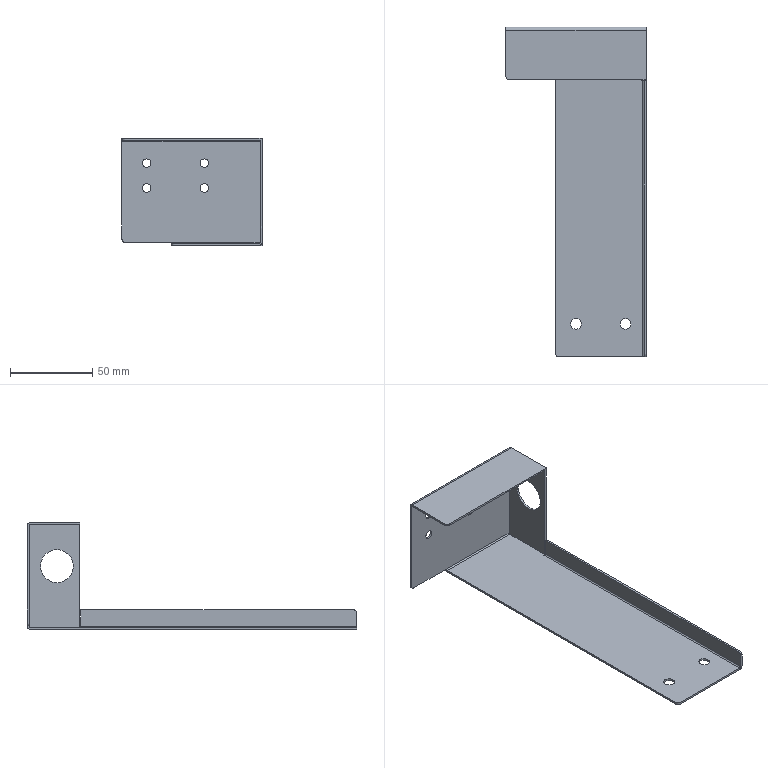Part | 1 solid | 50 faces | box 85 x 200 x 65 mm | volume 26532 mm3 | plane 26 | cylinder 24 | commonest cylinder face diameters 5.2 x8 4 x4 6.5 x4 1.473 x3 3.873 x3 20 x2
STEP:
#1=CARTESIAN_POINT('',(26.3,82.,27.3));
#2=VERTEX_POINT('',#1);
#3=CARTESIAN_POINT('',(26.3,82.,47.3));
#4=VERTEX_POINT('',#3);
#5=CARTESIAN_POINT('',(26.3,82.,37.3));
#6=DIRECTION('',(-1.,0.,0.));
#7=DIRECTION('',(0.,0.,1.));
#8=AXIS2_PLACEMENT_3D('',#5,#6,#7);
#9=CIRCLE('',#8,10.);
#10=EDGE_CURVE('',#2,#4,#9,.T.);
#11=ORIENTED_EDGE('',*,*,#10,.T.);
#12=CARTESIAN_POINT('',(27.5,82.,47.3));
#13=VERTEX_POINT('',#12);
#14=CARTESIAN_POINT('',(-57.5,82.,47.3));
#15=DIRECTION('',(1.,0.,0.));
#16=VECTOR('',#15,1000.);
#17=LINE('',#14,#16);
#18=EDGE_CURVE('',#4,#13,#17,.T.);
#19=ORIENTED_EDGE('',*,*,#18,.T.);
#20=CARTESIAN_POINT('',(27.5,82.,27.3));
#21=VERTEX_POINT('',#20);
#22=CARTESIAN_POINT('',(27.5,82.,37.3));
#23=DIRECTION('',(1.,0.,0.));
#24=DIRECTION('',(0.,0.,-1.));
#25=AXIS2_PLACEMENT_3D('',#22,#23,#24);
#26=CIRCLE('',#25,10.);
#27=EDGE_CURVE('',#13,#21,#26,.T.);
#28=ORIENTED_EDGE('',*,*,#27,.T.);
#29=CARTESIAN_POINT('',(-57.5,82.,27.3));
#30=DIRECTION('',(1.,0.,0.));
#31=VECTOR('',#30,1000.);
#32=LINE('',#29,#31);
#33=EDGE_CURVE('',#2,#21,#32,.T.);
#34=ORIENTED_EDGE('',*,*,#33,.F.);
#35=EDGE_LOOP('',(#11,#19,#28,#34));
#36=FACE_OUTER_BOUND('',#35,.T.);
#37=CARTESIAN_POINT('',(-57.5,82.,37.3));
#38=DIRECTION('',(1.,0.,0.));
#39=DIRECTION('',(0.,0.,-1.));
#40=AXIS2_PLACEMENT_3D('',#37,#38,#39);
#41=CYLINDRICAL_SURFACE('',#40,10.);
#42=ADVANCED_FACE('',(#36),#41,.F.);
#43=CARTESIAN_POINT('',(-7.5,98.8,46.2));
#44=VERTEX_POINT('',#43);
#45=CARTESIAN_POINT('',(-7.5,98.8,51.4));
#46=VERTEX_POINT('',#45);
#47=CARTESIAN_POINT('',(-7.5,98.8,48.8));
#48=DIRECTION('',(0.,1.,0.));
#49=DIRECTION('',(0.,0.,1.));
#50=AXIS2_PLACEMENT_3D('',#47,#48,#49);
#51=CIRCLE('',#50,2.6);
#52=EDGE_CURVE('',#44,#46,#51,.T.);
#53=ORIENTED_EDGE('',*,*,#52,.F.);
#54=CARTESIAN_POINT('',(-7.5,100.,46.2));
#55=VERTEX_POINT('',#54);
#56=CARTESIAN_POINT('',(-7.5,90.,46.2));
#57=DIRECTION('',(0.,1.,0.));
#58=VECTOR('',#57,1000.);
#59=LINE('',#56,#58);
#60=EDGE_CURVE('',#44,#55,#59,.T.);
#61=ORIENTED_EDGE('',*,*,#60,.T.);
#62=CARTESIAN_POINT('',(-7.5,100.,51.4));
#63=VERTEX_POINT('',#62);
#64=CARTESIAN_POINT('',(-7.5,100.,48.8));
#65=DIRECTION('',(0.,1.,0.));
#66=DIRECTION('',(0.,0.,1.));
#67=AXIS2_PLACEMENT_3D('',#64,#65,#66);
#68=CIRCLE('',#67,2.6);
#69=EDGE_CURVE('',#55,#63,#68,.T.);
#70=ORIENTED_EDGE('',*,*,#69,.T.);
#71=CARTESIAN_POINT('',(-7.5,90.,51.4));
#72=DIRECTION('',(0.,1.,0.));
#73=VECTOR('',#72,1000.);
#74=LINE('',#71,#73);
#75=EDGE_CURVE('',#46,#63,#74,.T.);
#76=ORIENTED_EDGE('',*,*,#75,.F.);
#77=EDGE_LOOP('',(#53,#61,#70,#76));
#78=FACE_OUTER_BOUND('',#77,.T.);
#79=CARTESIAN_POINT('',(-7.5,90.,48.8));
#80=DIRECTION('',(0.,1.,0.));
#81=DIRECTION('',(0.,0.,1.));
#82=AXIS2_PLACEMENT_3D('',#79,#80,#81);
#83=CYLINDRICAL_SURFACE('',#82,2.6);
#84=ADVANCED_FACE('',(#78),#83,.F.);
#85=CARTESIAN_POINT('',(-42.5,98.8,46.2));
#86=VERTEX_POINT('',#85);
#87=CARTESIAN_POINT('',(-42.5,98.8,51.4));
#88=VERTEX_POINT('',#87);
#89=CARTESIAN_POINT('',(-42.5,98.8,48.8));
#90=DIRECTION('',(0.,1.,0.));
#91=DIRECTION('',(0.,0.,1.));
#92=AXIS2_PLACEMENT_3D('',#89,#90,#91);
#93=CIRCLE('',#92,2.6);
#94=EDGE_CURVE('',#86,#88,#93,.T.);
#95=ORIENTED_EDGE('',*,*,#94,.F.);
#96=CARTESIAN_POINT('',(-42.5,100.,46.2));
#97=VERTEX_POINT('',#96);
#98=CARTESIAN_POINT('',(-42.5,90.,46.2));
#99=DIRECTION('',(0.,1.,0.));
#100=VECTOR('',#99,1000.);
#101=LINE('',#98,#100);
#102=EDGE_CURVE('',#86,#97,#101,.T.);
#103=ORIENTED_EDGE('',*,*,#102,.T.);
#104=CARTESIAN_POINT('',(-42.5,100.,51.4));
#105=VERTEX_POINT('',#104);
#106=CARTESIAN_POINT('',(-42.5,100.,48.8));
#107=DIRECTION('',(0.,1.,0.));
#108=DIRECTION('',(0.,0.,1.));
#109=AXIS2_PLACEMENT_3D('',#106,#107,#108);
#110=CIRCLE('',#109,2.6);
#111=EDGE_CURVE('',#97,#105,#110,.T.);
#112=ORIENTED_EDGE('',*,*,#111,.T.);
#113=CARTESIAN_POINT('',(-42.5,90.,51.4));
#114=DIRECTION('',(0.,1.,0.));
#115=VECTOR('',#114,1000.);
#116=LINE('',#113,#115);
#117=EDGE_CURVE('',#88,#105,#116,.T.);
#118=ORIENTED_EDGE('',*,*,#117,.F.);
#119=EDGE_LOOP('',(#95,#103,#112,#118));
#120=FACE_OUTER_BOUND('',#119,.T.);
#121=CARTESIAN_POINT('',(-42.5,90.,48.8));
#122=DIRECTION('',(0.,1.,0.));
#123=DIRECTION('',(0.,0.,1.));
#124=AXIS2_PLACEMENT_3D('',#121,#122,#123);
#125=CYLINDRICAL_SURFACE('',#124,2.6);
#126=ADVANCED_FACE('',(#120),#125,.F.);
#127=CARTESIAN_POINT('',(-42.5,98.8,31.2));
#128=VERTEX_POINT('',#127);
#129=CARTESIAN_POINT('',(-42.5,98.8,36.4));
#130=VERTEX_POINT('',#129);
#131=CARTESIAN_POINT('',(-42.5,98.8,33.8));
#132=DIRECTION('',(0.,1.,0.));
#133=DIRECTION('',(0.,0.,1.));
#134=AXIS2_PLACEMENT_3D('',#131,#132,#133);
#135=CIRCLE('',#134,2.6);
#136=EDGE_CURVE('',#128,#130,#135,.T.);
#137=ORIENTED_EDGE('',*,*,#136,.F.);
#138=CARTESIAN_POINT('',(-42.5,100.,31.2));
#139=VERTEX_POINT('',#138);
#140=CARTESIAN_POINT('',(-42.5,90.,31.2));
#141=DIRECTION('',(0.,1.,0.));
#142=VECTOR('',#141,1000.);
#143=LINE('',#140,#142);
#144=EDGE_CURVE('',#128,#139,#143,.T.);
#145=ORIENTED_EDGE('',*,*,#144,.T.);
#146=CARTESIAN_POINT('',(-42.5,100.,36.4));
#147=VERTEX_POINT('',#146);
#148=CARTESIAN_POINT('',(-42.5,100.,33.8));
#149=DIRECTION('',(0.,1.,0.));
#150=DIRECTION('',(0.,0.,1.));
#151=AXIS2_PLACEMENT_3D('',#148,#149,#150);
#152=CIRCLE('',#151,2.6);
#153=EDGE_CURVE('',#139,#147,#152,.T.);
#154=ORIENTED_EDGE('',*,*,#153,.T.);
#155=CARTESIAN_POINT('',(-42.5,90.,36.4));
#156=DIRECTION('',(0.,1.,0.));
#157=VECTOR('',#156,1000.);
#158=LINE('',#155,#157);
#159=EDGE_CURVE('',#130,#147,#158,.T.);
#160=ORIENTED_EDGE('',*,*,#159,.F.);
#161=EDGE_LOOP('',(#137,#145,#154,#160));
#162=FACE_OUTER_BOUND('',#161,.T.);
#163=CARTESIAN_POINT('',(-42.5,90.,33.8));
#164=DIRECTION('',(0.,1.,0.));
#165=DIRECTION('',(0.,0.,1.));
#166=AXIS2_PLACEMENT_3D('',#163,#164,#165);
#167=CYLINDRICAL_SURFACE('',#166,2.6);
#168=ADVANCED_FACE('',(#162),#167,.F.);
#169=CARTESIAN_POINT('',(-7.5,98.8,31.2));
#170=VERTEX_POINT('',#169);
#171=CARTESIAN_POINT('',(-7.5,98.8,36.4));
#172=VERTEX_POINT('',#171);
#173=CARTESIAN_POINT('',(-7.5,98.8,33.8));
#174=DIRECTION('',(0.,1.,0.));
#175=DIRECTION('',(0.,0.,1.));
#176=AXIS2_PLACEMENT_3D('',#173,#174,#175);
#177=CIRCLE('',#176,2.6);
#178=EDGE_CURVE('',#170,#172,#177,.T.);
#179=ORIENTED_EDGE('',*,*,#178,.F.);
#180=CARTESIAN_POINT('',(-7.5,100.,31.2));
#181=VERTEX_POINT('',#180);
#182=CARTESIAN_POINT('',(-7.5,90.,31.2));
#183=DIRECTION('',(0.,1.,0.));
#184=VECTOR('',#183,1000.);
#185=LINE('',#182,#184);
#186=EDGE_CURVE('',#170,#181,#185,.T.);
#187=ORIENTED_EDGE('',*,*,#186,.T.);
#188=CARTESIAN_POINT('',(-7.5,100.,36.4));
#189=VERTEX_POINT('',#188);
#190=CARTESIAN_POINT('',(-7.5,100.,33.8));
#191=DIRECTION('',(0.,1.,0.));
#192=DIRECTION('',(0.,0.,1.));
#193=AXIS2_PLACEMENT_3D('',#190,#191,#192);
#194=CIRCLE('',#193,2.6);
#195=EDGE_CURVE('',#181,#189,#194,.T.);
#196=ORIENTED_EDGE('',*,*,#195,.T.);
#197=CARTESIAN_POINT('',(-7.5,90.,36.4));
#198=DIRECTION('',(0.,1.,0.));
#199=VECTOR('',#198,1000.);
#200=LINE('',#197,#199);
#201=EDGE_CURVE('',#172,#189,#200,.T.);
#202=ORIENTED_EDGE('',*,*,#201,.F.);
#203=EDGE_LOOP('',(#179,#187,#196,#202));
#204=FACE_OUTER_BOUND('',#203,.T.);
#205=CARTESIAN_POINT('',(-7.5,90.,33.8));
#206=DIRECTION('',(0.,1.,0.));
#207=DIRECTION('',(0.,0.,1.));
#208=AXIS2_PLACEMENT_3D('',#205,#206,#207);
#209=CYLINDRICAL_SURFACE('',#208,2.6);
#210=ADVANCED_FACE('',(#204),#209,.F.);
#211=CARTESIAN_POINT('',(18.25,-80.,0.));
#212=VERTEX_POINT('',#211);
#213=CARTESIAN_POINT('',(11.75,-80.,0.));
#214=VERTEX_POINT('',#213);
#215=CARTESIAN_POINT('',(15.,-80.,0.));
#216=DIRECTION('',(0.,0.,-1.));
#217=DIRECTION('',(-1.,0.,0.));
#218=AXIS2_PLACEMENT_3D('',#215,#216,#217);
#219=CIRCLE('',#218,3.25);
#220=EDGE_CURVE('',#212,#214,#219,.T.);
#221=ORIENTED_EDGE('',*,*,#220,.F.);
#222=CARTESIAN_POINT('',(18.25,-80.,-1.2));
#223=VERTEX_POINT('',#222);
#224=CARTESIAN_POINT('',(18.25,-80.,8.8));
#225=DIRECTION('',(0.,0.,-1.));
#226=VECTOR('',#225,1000.);
#227=LINE('',#224,#226);
#228=EDGE_CURVE('',#212,#223,#227,.T.);
#229=ORIENTED_EDGE('',*,*,#228,.T.);
#230=CARTESIAN_POINT('',(11.75,-80.,-1.2));
#231=VERTEX_POINT('',#230);
#232=CARTESIAN_POINT('',(15.,-80.,-1.2));
#233=DIRECTION('',(0.,0.,-1.));
#234=DIRECTION('',(-1.,0.,0.));
#235=AXIS2_PLACEMENT_3D('',#232,#233,#234);
#236=CIRCLE('',#235,3.25);
#237=EDGE_CURVE('',#223,#231,#236,.T.);
#238=ORIENTED_EDGE('',*,*,#237,.T.);
#239=CARTESIAN_POINT('',(11.75,-80.,8.8));
#240=DIRECTION('',(0.,0.,-1.));
#241=VECTOR('',#240,1000.);
#242=LINE('',#239,#241);
#243=EDGE_CURVE('',#214,#231,#242,.T.);
#244=ORIENTED_EDGE('',*,*,#243,.F.);
#245=EDGE_LOOP('',(#221,#229,#238,#244));
#246=FACE_OUTER_BOUND('',#245,.T.);
#247=CARTESIAN_POINT('',(15.,-80.,8.8));
#248=DIRECTION('',(0.,0.,-1.));
#249=DIRECTION('',(-1.,0.,0.));
#250=AXIS2_PLACEMENT_3D('',#247,#248,#249);
#251=CYLINDRICAL_SURFACE('',#250,3.25);
#252=ADVANCED_FACE('',(#246),#251,.F.);
#253=CARTESIAN_POINT('',(-11.75,-80.,0.));
#254=VERTEX_POINT('',#253);
#255=CARTESIAN_POINT('',(-18.25,-80.,0.));
#256=VERTEX_POINT('',#255);
#257=CARTESIAN_POINT('',(-15.,-80.,0.));
#258=DIRECTION('',(0.,0.,-1.));
#259=DIRECTION('',(-1.,0.,0.));
#260=AXIS2_PLACEMENT_3D('',#257,#258,#259);
#261=CIRCLE('',#260,3.25);
#262=EDGE_CURVE('',#254,#256,#261,.T.);
#263=ORIENTED_EDGE('',*,*,#262,.F.);
#264=CARTESIAN_POINT('',(-11.75,-80.,-1.2));
#265=VERTEX_POINT('',#264);
#266=CARTESIAN_POINT('',(-11.75,-80.,8.8));
#267=DIRECTION('',(0.,0.,-1.));
#268=VECTOR('',#267,1000.);
#269=LINE('',#266,#268);
#270=EDGE_CURVE('',#254,#265,#269,.T.);
#271=ORIENTED_EDGE('',*,*,#270,.T.);
#272=CARTESIAN_POINT('',(-18.25,-80.,-1.2));
#273=VERTEX_POINT('',#272);
#274=CARTESIAN_POINT('',(-15.,-80.,-1.2));
#275=DIRECTION('',(0.,0.,-1.));
#276=DIRECTION('',(-1.,0.,0.));
#277=AXIS2_PLACEMENT_3D('',#274,#275,#276);
#278=CIRCLE('',#277,3.25);
#279=EDGE_CURVE('',#265,#273,#278,.T.);
#280=ORIENTED_EDGE('',*,*,#279,.T.);
#281=CARTESIAN_POINT('',(-18.25,-80.,8.8));
#282=DIRECTION('',(0.,0.,-1.));
#283=VECTOR('',#282,1000.);
#284=LINE('',#281,#283);
#285=EDGE_CURVE('',#256,#273,#284,.T.);
#286=ORIENTED_EDGE('',*,*,#285,.F.);
#287=EDGE_LOOP('',(#263,#271,#280,#286));
#288=FACE_OUTER_BOUND('',#287,.T.);
#289=CARTESIAN_POINT('',(-15.,-80.,8.8));
#290=DIRECTION('',(0.,0.,-1.));
#291=DIRECTION('',(-1.,0.,0.));
#292=AXIS2_PLACEMENT_3D('',#289,#290,#291);
#293=CYLINDRICAL_SURFACE('',#292,3.25);
#294=ADVANCED_FACE('',(#288),#293,.F.);
#295=CARTESIAN_POINT('',(-25.5,-100.,-1.2));
#296=VERTEX_POINT('',#295);
#297=CARTESIAN_POINT('',(25.563,-100.,-1.2));
#298=VERTEX_POINT('',#297);
#299=CARTESIAN_POINT('',(-27.5,-100.,-1.2));
#300=DIRECTION('',(1.,0.,0.));
#301=VECTOR('',#300,1000.);
#302=LINE('',#299,#301);
#303=EDGE_CURVE('',#296,#298,#302,.T.);
#304=ORIENTED_EDGE('',*,*,#303,.F.);
#305=CARTESIAN_POINT('',(-27.5,-98.,-1.2));
#306=VERTEX_POINT('',#305);
#307=CARTESIAN_POINT('',(-25.5,-98.,-1.2));
#308=DIRECTION('',(0.,0.,-1.));
#309=DIRECTION('',(-1.,0.,0.));
#310=AXIS2_PLACEMENT_3D('',#307,#308,#309);
#311=CIRCLE('',#310,2.);
#312=EDGE_CURVE('',#296,#306,#311,.T.);
#313=ORIENTED_EDGE('',*,*,#312,.T.);
#314=CARTESIAN_POINT('',(-27.5,98.063,-1.2));
#315=VERTEX_POINT('',#314);
#316=CARTESIAN_POINT('',(-27.5,-100.,-1.2));
#317=DIRECTION('',(0.,-1.,0.));
#318=VECTOR('',#317,1000.);
#319=LINE('',#316,#318);
#320=EDGE_CURVE('',#315,#306,#319,.T.);
#321=ORIENTED_EDGE('',*,*,#320,.F.);
#322=CARTESIAN_POINT('',(27.5,98.063,-1.2));
#323=VERTEX_POINT('',#322);
#324=CARTESIAN_POINT('',(-27.5,98.063,-1.2));
#325=DIRECTION('',(1.,0.,0.));
#326=VECTOR('',#325,1000.);
#327=LINE('',#324,#326);
#328=EDGE_CURVE('',#315,#323,#327,.T.);
#329=ORIENTED_EDGE('',*,*,#328,.T.);
#330=CARTESIAN_POINT('',(27.5,68.,-1.2));
#331=VERTEX_POINT('',#330);
#332=CARTESIAN_POINT('',(27.5,-100.,-1.2));
#333=DIRECTION('',(0.,1.,0.));
#334=VECTOR('',#333,1000.);
#335=LINE('',#332,#334);
#336=EDGE_CURVE('',#331,#323,#335,.T.);
#337=ORIENTED_EDGE('',*,*,#336,.F.);
#338=CARTESIAN_POINT('',(26.3,68.,-1.2));
#339=VERTEX_POINT('',#338);
#340=CARTESIAN_POINT('',(26.3,68.,-1.2));
#341=DIRECTION('',(1.,0.,0.));
#342=VECTOR('',#341,1000.);
#343=LINE('',#340,#342);
#344=EDGE_CURVE('',#339,#331,#343,.T.);
#345=ORIENTED_EDGE('',*,*,#344,.F.);
#346=CARTESIAN_POINT('',(26.3,68.2,-1.2));
#347=VERTEX_POINT('',#346);
#348=CARTESIAN_POINT('',(26.3,68.,-1.2));
#349=DIRECTION('',(0.,1.,0.));
#350=VECTOR('',#349,1000.);
#351=LINE('',#348,#350);
#352=EDGE_CURVE('',#339,#347,#351,.T.);
#353=ORIENTED_EDGE('',*,*,#352,.T.);
#354=CARTESIAN_POINT('',(24.963,68.2,-1.2));
#355=VERTEX_POINT('',#354);
#356=CARTESIAN_POINT('',(0.,68.2,-1.2));
#357=DIRECTION('',(-1.,0.,0.));
#358=VECTOR('',#357,1000.);
#359=LINE('',#356,#358);
#360=EDGE_CURVE('',#347,#355,#359,.T.);
#361=ORIENTED_EDGE('',*,*,#360,.T.);
#362=CARTESIAN_POINT('',(24.963,67.6,-1.2));
#363=VERTEX_POINT('',#362);
#364=CARTESIAN_POINT('',(24.963,0.,-1.2));
#365=DIRECTION('',(0.,-1.,0.));
#366=VECTOR('',#365,1000.);
#367=LINE('',#364,#366);
#368=EDGE_CURVE('',#355,#363,#367,.T.);
#369=ORIENTED_EDGE('',*,*,#368,.T.);
#370=CARTESIAN_POINT('',(25.563,67.6,-1.2));
#371=VERTEX_POINT('',#370);
#372=CARTESIAN_POINT('',(0.,67.6,-1.2));
#373=DIRECTION('',(1.,0.,0.));
#374=VECTOR('',#373,1000.);
#375=LINE('',#372,#374);
#376=EDGE_CURVE('',#363,#371,#375,.T.);
#377=ORIENTED_EDGE('',*,*,#376,.T.);
#378=CARTESIAN_POINT('',(25.563,67.6,-1.2));
#379=DIRECTION('',(0.,-1.,0.));
#380=VECTOR('',#379,1000.);
#381=LINE('',#378,#380);
#382=EDGE_CURVE('',#371,#298,#381,.T.);
#383=ORIENTED_EDGE('',*,*,#382,.T.);
#384=EDGE_LOOP('',(#304,#313,#321,#329,#337,#345,#353,#361,#369,#377,#383));
#385=FACE_OUTER_BOUND('',#384,.T.);
#386=CARTESIAN_POINT('',(15.,-80.,-1.2));
#387=DIRECTION('',(0.,0.,-1.));
#388=DIRECTION('',(-1.,0.,0.));
#389=AXIS2_PLACEMENT_3D('',#386,#387,#388);
#390=CIRCLE('',#389,3.25);
#391=EDGE_CURVE('',#231,#223,#390,.T.);
#392=ORIENTED_EDGE('',*,*,#391,.F.);
#393=ORIENTED_EDGE('',*,*,#237,.F.);
#394=EDGE_LOOP('',(#392,#393));
#395=FACE_BOUND('',#394,.T.);
#396=CARTESIAN_POINT('',(-15.,-80.,-1.2));
#397=DIRECTION('',(0.,0.,-1.));
#398=DIRECTION('',(-1.,0.,0.));
#399=AXIS2_PLACEMENT_3D('',#396,#397,#398);
#400=CIRCLE('',#399,3.25);
#401=EDGE_CURVE('',#273,#265,#400,.T.);
#402=ORIENTED_EDGE('',*,*,#401,.F.);
#403=ORIENTED_EDGE('',*,*,#279,.F.);
#404=EDGE_LOOP('',(#402,#403));
#405=FACE_BOUND('',#404,.T.);
#406=CARTESIAN_POINT('',(0.,0.,-1.2));
#407=DIRECTION('',(0.,0.,-1.));
#408=DIRECTION('',(-1.,0.,0.));
#409=AXIS2_PLACEMENT_3D('',#406,#407,#408);
#410=PLANE('',#409);
#411=ADVANCED_FACE('',(#385,#395,#405),#410,.T.);
#412=CARTESIAN_POINT('',(-15.,-80.,0.));
#413=DIRECTION('',(0.,0.,-1.));
#414=DIRECTION('',(-1.,0.,0.));
#415=AXIS2_PLACEMENT_3D('',#412,#413,#414);
#416=CIRCLE('',#415,3.25);
#417=EDGE_CURVE('',#256,#254,#416,.T.);
#418=ORIENTED_EDGE('',*,*,#417,.T.);
#419=ORIENTED_EDGE('',*,*,#262,.T.);
#420=EDGE_LOOP('',(#418,#419));
#421=FACE_BOUND('',#420,.T.);
#422=CARTESIAN_POINT('',(15.,-80.,0.));
#423=DIRECTION('',(0.,0.,-1.));
#424=DIRECTION('',(-1.,0.,0.));
#425=AXIS2_PLACEMENT_3D('',#422,#423,#424);
#426=CIRCLE('',#425,3.25);
#427=EDGE_CURVE('',#214,#212,#426,.T.);
#428=ORIENTED_EDGE('',*,*,#427,.T.);
#429=ORIENTED_EDGE('',*,*,#220,.T.);
#430=EDGE_LOOP('',(#428,#429));
#431=FACE_BOUND('',#430,.T.);
#432=CARTESIAN_POINT('',(-27.5,98.063,0.));
#433=VERTEX_POINT('',#432);
#434=CARTESIAN_POINT('',(-27.5,-98.,0.));
#435=VERTEX_POINT('',#434);
#436=CARTESIAN_POINT('',(-27.5,-100.,0.));
#437=DIRECTION('',(0.,-1.,0.));
#438=VECTOR('',#437,1000.);
#439=LINE('',#436,#438);
#440=EDGE_CURVE('',#433,#435,#439,.T.);
#441=ORIENTED_EDGE('',*,*,#440,.T.);
#442=CARTESIAN_POINT('',(-25.5,-100.,0.));
#443=VERTEX_POINT('',#442);
#444=CARTESIAN_POINT('',(-25.5,-98.,0.));
#445=DIRECTION('',(0.,0.,1.));
#446=DIRECTION('',(-1.,0.,0.));
#447=AXIS2_PLACEMENT_3D('',#444,#445,#446);
#448=CIRCLE('',#447,2.);
#449=EDGE_CURVE('',#435,#443,#448,.T.);
#450=ORIENTED_EDGE('',*,*,#449,.T.);
#451=CARTESIAN_POINT('',(25.563,-100.,0.));
#452=VERTEX_POINT('',#451);
#453=CARTESIAN_POINT('',(-27.5,-100.,0.));
#454=DIRECTION('',(1.,0.,0.));
#455=VECTOR('',#454,1000.);
#456=LINE('',#453,#455);
#457=EDGE_CURVE('',#443,#452,#456,.T.);
#458=ORIENTED_EDGE('',*,*,#457,.T.);
#459=CARTESIAN_POINT('',(25.563,67.6,0.));
#460=VERTEX_POINT('',#459);
#461=CARTESIAN_POINT('',(25.563,67.6,0.));
#462=DIRECTION('',(0.,-1.,0.));
#463=VECTOR('',#462,1000.);
#464=LINE('',#461,#463);
#465=EDGE_CURVE('',#460,#452,#464,.T.);
#466=ORIENTED_EDGE('',*,*,#465,.F.);
#467=CARTESIAN_POINT('',(24.963,67.6,0.));
#468=VERTEX_POINT('',#467);
#469=CARTESIAN_POINT('',(24.963,67.6,0.));
#470=DIRECTION('',(1.,0.,0.));
#471=VECTOR('',#470,1000.);
#472=LINE('',#469,#471);
#473=EDGE_CURVE('',#468,#460,#472,.T.);
#474=ORIENTED_EDGE('',*,*,#473,.F.);
#475=CARTESIAN_POINT('',(24.963,68.2,0.));
#476=VERTEX_POINT('',#475);
#477=CARTESIAN_POINT('',(24.963,68.2,0.));
#478=DIRECTION('',(0.,-1.,0.));
#479=VECTOR('',#478,1000.);
#480=LINE('',#477,#479);
#481=EDGE_CURVE('',#476,#468,#480,.T.);
#482=ORIENTED_EDGE('',*,*,#481,.F.);
#483=CARTESIAN_POINT('',(26.3,68.2,0.));
#484=VERTEX_POINT('',#483);
#485=CARTESIAN_POINT('',(27.5,68.2,0.));
#486=DIRECTION('',(-1.,0.,0.));
#487=VECTOR('',#486,1000.);
#488=LINE('',#485,#487);
#489=EDGE_CURVE('',#484,#476,#488,.T.);
#490=ORIENTED_EDGE('',*,*,#489,.F.);
#491=CARTESIAN_POINT('',(26.3,98.063,0.));
#492=VERTEX_POINT('',#491);
#493=CARTESIAN_POINT('',(26.3,0.,0.));
#494=DIRECTION('',(0.,1.,0.));
#495=VECTOR('',#494,1000.);
#496=LINE('',#493,#495);
#497=EDGE_CURVE('',#484,#492,#496,.T.);
#498=ORIENTED_EDGE('',*,*,#497,.T.);
#499=CARTESIAN_POINT('',(-27.5,98.063,0.));
#500=DIRECTION('',(1.,0.,0.));
#501=VECTOR('',#500,1000.);
#502=LINE('',#499,#501);
#503=EDGE_CURVE('',#433,#492,#502,.T.);
#504=ORIENTED_EDGE('',*,*,#503,.F.);
#505=EDGE_LOOP('',(#441,#450,#458,#466,#474,#482,#490,#498,#504));
#506=FACE_OUTER_BOUND('',#505,.T.);
#507=CARTESIAN_POINT('',(0.,0.,0.));
#508=DIRECTION('',(0.,0.,-1.));
#509=DIRECTION('',(-1.,0.,0.));
#510=AXIS2_PLACEMENT_3D('',#507,#508,#509);
#511=PLANE('',#510);
#512=ADVANCED_FACE('',(#421,#431,#506),#511,.F.);
#513=CARTESIAN_POINT('',(-57.5,100.,61.863));
#514=VERTEX_POINT('',#513);
#515=CARTESIAN_POINT('',(-57.5,100.,2.737));
#516=VERTEX_POINT('',#515);
#517=CARTESIAN_POINT('',(-57.5,100.,0.));
#518=DIRECTION('',(0.,0.,-1.));
#519=VECTOR('',#518,1000.);
#520=LINE('',#517,#519);
#521=EDGE_CURVE('',#514,#516,#520,.T.);
#522=ORIENTED_EDGE('',*,*,#521,.T.);
#523=CARTESIAN_POINT('',(-57.5,98.8,2.737));
#524=VERTEX_POINT('',#523);
#525=CARTESIAN_POINT('',(-57.5,100.,2.737));
#526=DIRECTION('',(0.,-1.,0.));
#527=VECTOR('',#526,1000.);
#528=LINE('',#525,#527);
#529=EDGE_CURVE('',#516,#524,#528,.T.);
#530=ORIENTED_EDGE('',*,*,#529,.T.);
#531=CARTESIAN_POINT('',(-57.5,98.8,61.863));
#532=VERTEX_POINT('',#531);
#533=CARTESIAN_POINT('',(-57.5,98.8,0.));
#534=DIRECTION('',(0.,0.,-1.));
#535=VECTOR('',#534,1000.);
#536=LINE('',#533,#535);
#537=EDGE_CURVE('',#532,#524,#536,.T.);
#538=ORIENTED_EDGE('',*,*,#537,.F.);
#539=CARTESIAN_POINT('',(-57.5,98.8,61.863));
#540=DIRECTION('',(0.,1.,0.));
#541=VECTOR('',#540,1000.);
#542=LINE('',#539,#541);
#543=EDGE_CURVE('',#532,#514,#542,.T.);
#544=ORIENTED_EDGE('',*,*,#543,.T.);
#545=EDGE_LOOP('',(#522,#530,#538,#544));
#546=FACE_OUTER_BOUND('',#545,.T.);
#547=CARTESIAN_POINT('',(-57.5,100.,0.));
#548=DIRECTION('',(-1.,0.,0.));
#549=DIRECTION('',(0.,0.,1.));
#550=AXIS2_PLACEMENT_3D('',#547,#548,#549);
#551=PLANE('',#550);
#552=ADVANCED_FACE('',(#546),#551,.T.);
#553=CARTESIAN_POINT('',(-27.5,100.,0.7366));
#554=VERTEX_POINT('',#553);
#555=CARTESIAN_POINT('',(-55.5,100.,0.7366));
#556=VERTEX_POINT('',#555);
#557=CARTESIAN_POINT('',(0.,100.,0.7366));
#558=DIRECTION('',(-1.,0.,0.));
#559=VECTOR('',#558,1000.);
#560=LINE('',#557,#559);
#561=EDGE_CURVE('',#554,#556,#560,.T.);
#562=ORIENTED_EDGE('',*,*,#561,.T.);
#563=CARTESIAN_POINT('',(-55.5,100.,2.737));
#564=DIRECTION('',(0.,1.,0.));
#565=DIRECTION('',(0.,0.,1.));
#566=AXIS2_PLACEMENT_3D('',#563,#564,#565);
#567=CIRCLE('',#566,2.);
#568=EDGE_CURVE('',#556,#516,#567,.T.);
#569=ORIENTED_EDGE('',*,*,#568,.T.);
#570=ORIENTED_EDGE('',*,*,#521,.F.);
#571=CARTESIAN_POINT('',(27.5,100.,61.863));
#572=VERTEX_POINT('',#571);
#573=CARTESIAN_POINT('',(-57.5,100.,61.863));
#574=DIRECTION('',(1.,0.,0.));
#575=VECTOR('',#574,1000.);
#576=LINE('',#573,#575);
#577=EDGE_CURVE('',#514,#572,#576,.T.);
#578=ORIENTED_EDGE('',*,*,#577,.T.);
#579=CARTESIAN_POINT('',(27.5,100.,0.7366));
#580=VERTEX_POINT('',#579);
#581=CARTESIAN_POINT('',(27.5,100.,63.8));
#582=DIRECTION('',(0.,0.,1.));
#583=VECTOR('',#582,1000.);
#584=LINE('',#581,#583);
#585=EDGE_CURVE('',#580,#572,#584,.T.);
#586=ORIENTED_EDGE('',*,*,#585,.F.);
#587=CARTESIAN_POINT('',(0.,100.,0.7366));
#588=DIRECTION('',(-1.,0.,0.));
#589=VECTOR('',#588,1000.);
#590=LINE('',#587,#589);
#591=EDGE_CURVE('',#580,#554,#590,.T.);
#592=ORIENTED_EDGE('',*,*,#591,.T.);
#593=EDGE_LOOP('',(#562,#569,#570,#578,#586,#592));
#594=FACE_OUTER_BOUND('',#593,.T.);
#595=CARTESIAN_POINT('',(-7.5,100.,48.8));
#596=DIRECTION('',(0.,1.,0.));
#597=DIRECTION('',(0.,0.,1.));
#598=AXIS2_PLACEMENT_3D('',#595,#596,#597);
#599=CIRCLE('',#598,2.6);
#600=EDGE_CURVE('',#63,#55,#599,.T.);
#601=ORIENTED_EDGE('',*,*,#600,.F.);
#602=ORIENTED_EDGE('',*,*,#69,.F.);
#603=EDGE_LOOP('',(#601,#602));
#604=FACE_BOUND('',#603,.T.);
#605=CARTESIAN_POINT('',(-42.5,100.,48.8));
#606=DIRECTION('',(0.,1.,0.));
#607=DIRECTION('',(0.,0.,1.));
#608=AXIS2_PLACEMENT_3D('',#605,#606,#607);
#609=CIRCLE('',#608,2.6);
#610=EDGE_CURVE('',#105,#97,#609,.T.);
#611=ORIENTED_EDGE('',*,*,#610,.F.);
#612=ORIENTED_EDGE('',*,*,#111,.F.);
#613=EDGE_LOOP('',(#611,#612));
#614=FACE_BOUND('',#613,.T.);
#615=CARTESIAN_POINT('',(-42.5,100.,33.8));
#616=DIRECTION('',(0.,1.,0.));
#617=DIRECTION('',(0.,0.,1.));
#618=AXIS2_PLACEMENT_3D('',#615,#616,#617);
#619=CIRCLE('',#618,2.6);
#620=EDGE_CURVE('',#147,#139,#619,.T.);
#621=ORIENTED_EDGE('',*,*,#620,.F.);
#622=ORIENTED_EDGE('',*,*,#153,.F.);
#623=EDGE_LOOP('',(#621,#622));
#624=FACE_BOUND('',#623,.T.);
#625=CARTESIAN_POINT('',(-7.5,100.,33.8));
#626=DIRECTION('',(0.,1.,0.));
#627=DIRECTION('',(0.,0.,1.));
#628=AXIS2_PLACEMENT_3D('',#625,#626,#627);
#629=CIRCLE('',#628,2.6);
#630=EDGE_CURVE('',#189,#181,#629,.T.);
#631=ORIENTED_EDGE('',*,*,#630,.F.);
#632=ORIENTED_EDGE('',*,*,#195,.F.);
#633=EDGE_LOOP('',(#631,#632));
#634=FACE_BOUND('',#633,.T.);
#635=CARTESIAN_POINT('',(0.,100.,0.));
#636=DIRECTION('',(0.,1.,0.));
#637=DIRECTION('',(0.,0.,1.));
#638=AXIS2_PLACEMENT_3D('',#635,#636,#637);
#639=PLANE('',#638);
#640=ADVANCED_FACE('',(#594,#604,#614,#624,#634),#639,.T.);
#641=CARTESIAN_POINT('',(-7.5,98.8,48.8));
#642=DIRECTION('',(0.,1.,0.));
#643=DIRECTION('',(0.,0.,1.));
#644=AXIS2_PLACEMENT_3D('',#641,#642,#643);
#645=CIRCLE('',#644,2.6);
#646=EDGE_CURVE('',#46,#44,#645,.T.);
#647=ORIENTED_EDGE('',*,*,#646,.T.);
#648=ORIENTED_EDGE('',*,*,#52,.T.);
#649=EDGE_LOOP('',(#647,#648));
#650=FACE_BOUND('',#649,.T.);
#651=CARTESIAN_POINT('',(-42.5,98.8,48.8));
#652=DIRECTION('',(0.,1.,0.));
#653=DIRECTION('',(0.,0.,1.));
#654=AXIS2_PLACEMENT_3D('',#651,#652,#653);
#655=CIRCLE('',#654,2.6);
#656=EDGE_CURVE('',#88,#86,#655,.T.);
#657=ORIENTED_EDGE('',*,*,#656,.T.);
#658=ORIENTED_EDGE('',*,*,#94,.T.);
#659=EDGE_LOOP('',(#657,#658));
#660=FACE_BOUND('',#659,.T.);
#661=CARTESIAN_POINT('',(-42.5,98.8,33.8));
#662=DIRECTION('',(0.,1.,0.));
#663=DIRECTION('',(0.,0.,1.));
#664=AXIS2_PLACEMENT_3D('',#661,#662,#663);
#665=CIRCLE('',#664,2.6);
#666=EDGE_CURVE('',#130,#128,#665,.T.);
#667=ORIENTED_EDGE('',*,*,#666,.T.);
#668=ORIENTED_EDGE('',*,*,#136,.T.);
#669=EDGE_LOOP('',(#667,#668));
#670=FACE_BOUND('',#669,.T.);
#671=CARTESIAN_POINT('',(-7.5,98.8,33.8));
#672=DIRECTION('',(0.,1.,0.));
#673=DIRECTION('',(0.,0.,1.));
#674=AXIS2_PLACEMENT_3D('',#671,#672,#673);
#675=CIRCLE('',#674,2.6);
#676=EDGE_CURVE('',#172,#170,#675,.T.);
#677=ORIENTED_EDGE('',*,*,#676,.T.);
#678=ORIENTED_EDGE('',*,*,#178,.T.);
#679=EDGE_LOOP('',(#677,#678));
#680=FACE_BOUND('',#679,.T.);
#681=ORIENTED_EDGE('',*,*,#537,.T.);
#682=CARTESIAN_POINT('',(-55.5,98.8,0.7366));
#683=VERTEX_POINT('',#682);
#684=CARTESIAN_POINT('',(-55.5,98.8,2.737));
#685=DIRECTION('',(0.,-1.,0.));
#686=DIRECTION('',(0.,0.,1.));
#687=AXIS2_PLACEMENT_3D('',#684,#685,#686);
#688=CIRCLE('',#687,2.);
#689=EDGE_CURVE('',#524,#683,#688,.T.);
#690=ORIENTED_EDGE('',*,*,#689,.T.);
#691=CARTESIAN_POINT('',(-27.5,98.8,0.7366));
#692=VERTEX_POINT('',#691);
#693=CARTESIAN_POINT('',(27.5,98.8,0.7366));
#694=DIRECTION('',(-1.,0.,0.));
#695=VECTOR('',#694,1000.);
#696=LINE('',#693,#695);
#697=EDGE_CURVE('',#692,#683,#696,.T.);
#698=ORIENTED_EDGE('',*,*,#697,.F.);
#699=CARTESIAN_POINT('',(26.3,98.8,0.7366));
#700=VERTEX_POINT('',#699);
#701=CARTESIAN_POINT('',(27.5,98.8,0.7366));
#702=DIRECTION('',(-1.,0.,0.));
#703=VECTOR('',#702,1000.);
#704=LINE('',#701,#703);
#705=EDGE_CURVE('',#700,#692,#704,.T.);
#706=ORIENTED_EDGE('',*,*,#705,.F.);
#707=CARTESIAN_POINT('',(26.3,98.8,61.863));
#708=VERTEX_POINT('',#707);
#709=CARTESIAN_POINT('',(26.3,98.8,0.));
#710=DIRECTION('',(0.,0.,1.));
#711=VECTOR('',#710,1000.);
#712=LINE('',#709,#711);
#713=EDGE_CURVE('',#700,#708,#712,.T.);
#714=ORIENTED_EDGE('',*,*,#713,.T.);
#715=CARTESIAN_POINT('',(-57.5,98.8,61.863));
#716=DIRECTION('',(1.,0.,0.));
#717=VECTOR('',#716,1000.);
#718=LINE('',#715,#717);
#719=EDGE_CURVE('',#532,#708,#718,.T.);
#720=ORIENTED_EDGE('',*,*,#719,.F.);
#721=EDGE_LOOP('',(#681,#690,#698,#706,#714,#720));
#722=FACE_OUTER_BOUND('',#721,.T.);
#723=CARTESIAN_POINT('',(0.,98.8,0.));
#724=DIRECTION('',(0.,1.,0.));
#725=DIRECTION('',(0.,0.,1.));
#726=AXIS2_PLACEMENT_3D('',#723,#724,#725);
#727=PLANE('',#726);
#728=ADVANCED_FACE('',(#650,#660,#670,#680,#722),#727,.F.);
#729=ORIENTED_EDGE('',*,*,#320,.T.);
#730=CARTESIAN_POINT('',(-27.5,-98.,-1.2));
#731=DIRECTION('',(0.,0.,1.));
#732=VECTOR('',#731,1000.);
#733=LINE('',#730,#732);
#734=EDGE_CURVE('',#306,#435,#733,.T.);
#735=ORIENTED_EDGE('',*,*,#734,.T.);
#736=ORIENTED_EDGE('',*,*,#440,.F.);
#737=CARTESIAN_POINT('',(-27.5,98.063,0.));
#738=DIRECTION('',(0.,0.,-1.));
#739=VECTOR('',#738,1000.);
#740=LINE('',#737,#739);
#741=EDGE_CURVE('',#433,#315,#740,.T.);
#742=ORIENTED_EDGE('',*,*,#741,.T.);
#743=EDGE_LOOP('',(#729,#735,#736,#742));
#744=FACE_OUTER_BOUND('',#743,.T.);
#745=CARTESIAN_POINT('',(-27.5,-100.,-1.2));
#746=DIRECTION('',(-1.,0.,0.));
#747=DIRECTION('',(0.,0.,1.));
#748=AXIS2_PLACEMENT_3D('',#745,#746,#747);
#749=PLANE('',#748);
#750=ADVANCED_FACE('',(#744),#749,.T.);
#751=ORIENTED_EDGE('',*,*,#457,.F.);
#752=CARTESIAN_POINT('',(-25.5,-100.,-1.2));
#753=DIRECTION('',(0.,0.,-1.));
#754=VECTOR('',#753,1000.);
#755=LINE('',#752,#754);
#756=EDGE_CURVE('',#443,#296,#755,.T.);
#757=ORIENTED_EDGE('',*,*,#756,.T.);
#758=ORIENTED_EDGE('',*,*,#303,.T.);
#759=CARTESIAN_POINT('',(25.563,-100.,0.));
#760=DIRECTION('',(0.,0.,-1.));
#761=VECTOR('',#760,1000.);
#762=LINE('',#759,#761);
#763=EDGE_CURVE('',#452,#298,#762,.T.);
#764=ORIENTED_EDGE('',*,*,#763,.F.);
#765=EDGE_LOOP('',(#751,#757,#758,#764));
#766=FACE_OUTER_BOUND('',#765,.T.);
#767=CARTESIAN_POINT('',(-27.5,-100.,-1.2));
#768=DIRECTION('',(0.,-1.,0.));
#769=DIRECTION('',(0.,0.,-1.));
#770=AXIS2_PLACEMENT_3D('',#767,#768,#769);
#771=PLANE('',#770);
#772=ADVANCED_FACE('',(#766),#771,.T.);
#773=CARTESIAN_POINT('',(27.5,98.063,63.8));
#774=VERTEX_POINT('',#773);
#775=CARTESIAN_POINT('',(27.5,98.063,61.863));
#776=DIRECTION('',(1.,0.,0.));
#777=DIRECTION('',(0.,0.,1.));
#778=AXIS2_PLACEMENT_3D('',#775,#776,#777);
#779=CIRCLE('',#778,1.937);
#780=EDGE_CURVE('',#572,#774,#779,.T.);
#781=ORIENTED_EDGE('',*,*,#780,.T.);
#782=CARTESIAN_POINT('',(27.5,68.,63.8));
#783=VERTEX_POINT('',#782);
#784=CARTESIAN_POINT('',(27.5,68.,63.8));
#785=DIRECTION('',(0.,-1.,0.));
#786=VECTOR('',#785,1000.);
#787=LINE('',#784,#786);
#788=EDGE_CURVE('',#774,#783,#787,.T.);
#789=ORIENTED_EDGE('',*,*,#788,.T.);
#790=CARTESIAN_POINT('',(27.5,68.,63.8));
#791=DIRECTION('',(0.,0.,-1.));
#792=VECTOR('',#791,1000.);
#793=LINE('',#790,#792);
#794=EDGE_CURVE('',#783,#331,#793,.T.);
#795=ORIENTED_EDGE('',*,*,#794,.T.);
#796=ORIENTED_EDGE('',*,*,#336,.T.);
#797=CARTESIAN_POINT('',(27.5,98.063,0.7366));
#798=DIRECTION('',(1.,0.,0.));
#799=DIRECTION('',(0.,0.,1.));
#800=AXIS2_PLACEMENT_3D('',#797,#798,#799);
#801=CIRCLE('',#800,1.937);
#802=EDGE_CURVE('',#323,#580,#801,.T.);
#803=ORIENTED_EDGE('',*,*,#802,.T.);
#804=ORIENTED_EDGE('',*,*,#585,.T.);
#805=EDGE_LOOP('',(#781,#789,#795,#796,#803,#804));
#806=FACE_OUTER_BOUND('',#805,.T.);
#807=CARTESIAN_POINT('',(27.5,82.,37.3));
#808=DIRECTION('',(1.,0.,0.));
#809=DIRECTION('',(0.,0.,-1.));
#810=AXIS2_PLACEMENT_3D('',#807,#808,#809);
#811=CIRCLE('',#810,10.);
#812=EDGE_CURVE('',#21,#13,#811,.T.);
#813=ORIENTED_EDGE('',*,*,#812,.F.);
#814=ORIENTED_EDGE('',*,*,#27,.F.);
#815=EDGE_LOOP('',(#813,#814));
#816=FACE_BOUND('',#815,.T.);
#817=CARTESIAN_POINT('',(27.5,98.063,0.7366));
#818=DIRECTION('',(1.,0.,0.));
#819=DIRECTION('',(0.,0.,-1.));
#820=AXIS2_PLACEMENT_3D('',#817,#818,#819);
#821=PLANE('',#820);
#822=ADVANCED_FACE('',(#806,#816),#821,.T.);
#823=CARTESIAN_POINT('',(-27.5,98.063,0.7366));
#824=DIRECTION('',(-1.,0.,0.));
#825=DIRECTION('',(0.,0.,1.));
#826=AXIS2_PLACEMENT_3D('',#823,#824,#825);
#827=CIRCLE('',#826,0.7366);
#828=EDGE_CURVE('',#692,#433,#827,.T.);
#829=ORIENTED_EDGE('',*,*,#828,.F.);
#830=CARTESIAN_POINT('',(-27.5,98.8,0.7366));
#831=DIRECTION('',(0.,1.,0.));
#832=VECTOR('',#831,1000.);
#833=LINE('',#830,#832);
#834=EDGE_CURVE('',#692,#554,#833,.T.);
#835=ORIENTED_EDGE('',*,*,#834,.T.);
#836=CARTESIAN_POINT('',(-27.5,98.063,0.7366));
#837=DIRECTION('',(-1.,0.,0.));
#838=DIRECTION('',(0.,0.,1.));
#839=AXIS2_PLACEMENT_3D('',#836,#837,#838);
#840=CIRCLE('',#839,1.937);
#841=EDGE_CURVE('',#554,#315,#840,.T.);
#842=ORIENTED_EDGE('',*,*,#841,.T.);
#843=ORIENTED_EDGE('',*,*,#741,.F.);
#844=EDGE_LOOP('',(#829,#835,#842,#843));
#845=FACE_OUTER_BOUND('',#844,.T.);
#846=CARTESIAN_POINT('',(-27.5,98.063,0.7366));
#847=DIRECTION('',(1.,0.,0.));
#848=DIRECTION('',(0.,0.,-1.));
#849=AXIS2_PLACEMENT_3D('',#846,#847,#848);
#850=PLANE('',#849);
#851=ADVANCED_FACE('',(#845),#850,.F.);
#852=ORIENTED_EDGE('',*,*,#328,.F.);
#853=ORIENTED_EDGE('',*,*,#841,.F.);
#854=ORIENTED_EDGE('',*,*,#591,.F.);
#855=ORIENTED_EDGE('',*,*,#802,.F.);
#856=EDGE_LOOP('',(#852,#853,#854,#855));
#857=FACE_OUTER_BOUND('',#856,.T.);
#858=CARTESIAN_POINT('',(-27.5,98.063,0.7366));
#859=DIRECTION('',(-1.,0.,0.));
#860=DIRECTION('',(0.,1.,0.));
#861=AXIS2_PLACEMENT_3D('',#858,#859,#860);
#862=CYLINDRICAL_SURFACE('',#861,1.937);
#863=ADVANCED_FACE('',(#857),#862,.T.);
#864=ORIENTED_EDGE('',*,*,#503,.T.);
#865=CARTESIAN_POINT('',(26.3,98.063,0.7366));
#866=DIRECTION('',(1.,0.,0.));
#867=DIRECTION('',(0.,0.,1.));
#868=AXIS2_PLACEMENT_3D('',#865,#866,#867);
#869=CIRCLE('',#868,0.7366);
#870=EDGE_CURVE('',#492,#700,#869,.T.);
#871=ORIENTED_EDGE('',*,*,#870,.T.);
#872=ORIENTED_EDGE('',*,*,#705,.T.);
#873=ORIENTED_EDGE('',*,*,#828,.T.);
#874=EDGE_LOOP('',(#864,#871,#872,#873));
#875=FACE_OUTER_BOUND('',#874,.T.);
#876=CARTESIAN_POINT('',(-27.5,98.063,0.7366));
#877=DIRECTION('',(-1.,0.,0.));
#878=DIRECTION('',(0.,1.,0.));
#879=AXIS2_PLACEMENT_3D('',#876,#877,#878);
#880=CYLINDRICAL_SURFACE('',#879,0.7366);
#881=ADVANCED_FACE('',(#875),#880,.F.);
#882=ORIENTED_EDGE('',*,*,#697,.T.);
#883=CARTESIAN_POINT('',(-55.5,98.8,0.7366));
#884=DIRECTION('',(0.,1.,0.));
#885=VECTOR('',#884,1000.);
#886=LINE('',#883,#885);
#887=EDGE_CURVE('',#683,#556,#886,.T.);
#888=ORIENTED_EDGE('',*,*,#887,.T.);
#889=ORIENTED_EDGE('',*,*,#561,.F.);
#890=ORIENTED_EDGE('',*,*,#834,.F.);
#891=EDGE_LOOP('',(#882,#888,#889,#890));
#892=FACE_OUTER_BOUND('',#891,.T.);
#893=CARTESIAN_POINT('',(27.5,98.8,0.7366));
#894=DIRECTION('',(0.,0.,-1.));
#895=DIRECTION('',(0.,1.,0.));
#896=AXIS2_PLACEMENT_3D('',#893,#894,#895);
#897=PLANE('',#896);
#898=ADVANCED_FACE('',(#892),#897,.T.);
#899=CARTESIAN_POINT('',(-57.5,98.063,62.6));
#900=VERTEX_POINT('',#899);
#901=CARTESIAN_POINT('',(-57.5,98.063,61.863));
#902=DIRECTION('',(-1.,0.,0.));
#903=DIRECTION('',(0.,0.,1.));
#904=AXIS2_PLACEMENT_3D('',#901,#902,#903);
#905=CIRCLE('',#904,0.7366);
#906=EDGE_CURVE('',#900,#532,#905,.T.);
#907=ORIENTED_EDGE('',*,*,#906,.F.);
#908=CARTESIAN_POINT('',(-57.5,98.063,63.8));
#909=VERTEX_POINT('',#908);
#910=CARTESIAN_POINT('',(-57.5,98.063,62.6));
#911=DIRECTION('',(0.,0.,1.));
#912=VECTOR('',#911,1000.);
#913=LINE('',#910,#912);
#914=EDGE_CURVE('',#900,#909,#913,.T.);
#915=ORIENTED_EDGE('',*,*,#914,.T.);
#916=CARTESIAN_POINT('',(-57.5,98.063,61.863));
#917=DIRECTION('',(-1.,0.,0.));
#918=DIRECTION('',(0.,0.,1.));
#919=AXIS2_PLACEMENT_3D('',#916,#917,#918);
#920=CIRCLE('',#919,1.937);
#921=EDGE_CURVE('',#909,#514,#920,.T.);
#922=ORIENTED_EDGE('',*,*,#921,.T.);
#923=ORIENTED_EDGE('',*,*,#543,.F.);
#924=EDGE_LOOP('',(#907,#915,#922,#923));
#925=FACE_OUTER_BOUND('',#924,.T.);
#926=CARTESIAN_POINT('',(-57.5,98.063,61.863));
#927=DIRECTION('',(1.,0.,0.));
#928=DIRECTION('',(0.,0.,-1.));
#929=AXIS2_PLACEMENT_3D('',#926,#927,#928);
#930=PLANE('',#929);
#931=ADVANCED_FACE('',(#925),#930,.F.);
#932=ORIENTED_EDGE('',*,*,#577,.F.);
#933=ORIENTED_EDGE('',*,*,#921,.F.);
#934=CARTESIAN_POINT('',(0.,98.063,63.8));
#935=DIRECTION('',(-1.,0.,0.));
#936=VECTOR('',#935,1000.);
#937=LINE('',#934,#936);
#938=EDGE_CURVE('',#774,#909,#937,.T.);
#939=ORIENTED_EDGE('',*,*,#938,.F.);
#940=ORIENTED_EDGE('',*,*,#780,.F.);
#941=EDGE_LOOP('',(#932,#933,#939,#940));
#942=FACE_OUTER_BOUND('',#941,.T.);
#943=CARTESIAN_POINT('',(-57.5,98.063,61.863));
#944=DIRECTION('',(-1.,0.,0.));
#945=DIRECTION('',(0.,0.,1.));
#946=AXIS2_PLACEMENT_3D('',#943,#944,#945);
#947=CYLINDRICAL_SURFACE('',#946,1.937);
#948=ADVANCED_FACE('',(#942),#947,.T.);
#949=ORIENTED_EDGE('',*,*,#719,.T.);
#950=CARTESIAN_POINT('',(26.3,98.063,62.6));
#951=VERTEX_POINT('',#950);
#952=CARTESIAN_POINT('',(26.3,98.063,61.863));
#953=DIRECTION('',(1.,0.,0.));
#954=DIRECTION('',(0.,0.,1.));
#955=AXIS2_PLACEMENT_3D('',#952,#953,#954);
#956=CIRCLE('',#955,0.7366);
#957=EDGE_CURVE('',#708,#951,#956,.T.);
#958=ORIENTED_EDGE('',*,*,#957,.T.);
#959=CARTESIAN_POINT('',(27.5,98.063,62.6));
#960=DIRECTION('',(-1.,0.,0.));
#961=VECTOR('',#960,1000.);
#962=LINE('',#959,#961);
#963=EDGE_CURVE('',#951,#900,#962,.T.);
#964=ORIENTED_EDGE('',*,*,#963,.T.);
#965=ORIENTED_EDGE('',*,*,#906,.T.);
#966=EDGE_LOOP('',(#949,#958,#964,#965));
#967=FACE_OUTER_BOUND('',#966,.T.);
#968=CARTESIAN_POINT('',(-57.5,98.063,61.863));
#969=DIRECTION('',(-1.,0.,0.));
#970=DIRECTION('',(0.,0.,1.));
#971=AXIS2_PLACEMENT_3D('',#968,#969,#970);
#972=CYLINDRICAL_SURFACE('',#971,0.7366);
#973=ADVANCED_FACE('',(#967),#972,.F.);
#974=CARTESIAN_POINT('',(-57.5,70.,62.6));
#975=VERTEX_POINT('',#974);
#976=CARTESIAN_POINT('',(-57.5,0.,62.6));
#977=DIRECTION('',(0.,1.,0.));
#978=VECTOR('',#977,1000.);
#979=LINE('',#976,#978);
#980=EDGE_CURVE('',#975,#900,#979,.T.);
#981=ORIENTED_EDGE('',*,*,#980,.F.);
#982=CARTESIAN_POINT('',(-57.5,70.,63.8));
#983=VERTEX_POINT('',#982);
#984=CARTESIAN_POINT('',(-57.5,70.,63.8));
#985=DIRECTION('',(0.,0.,1.));
#986=VECTOR('',#985,1000.);
#987=LINE('',#984,#986);
#988=EDGE_CURVE('',#975,#983,#987,.T.);
#989=ORIENTED_EDGE('',*,*,#988,.T.);
#990=CARTESIAN_POINT('',(-57.5,98.8,63.8));
#991=DIRECTION('',(0.,1.,0.));
#992=VECTOR('',#991,1000.);
#993=LINE('',#990,#992);
#994=EDGE_CURVE('',#983,#909,#993,.T.);
#995=ORIENTED_EDGE('',*,*,#994,.T.);
#996=ORIENTED_EDGE('',*,*,#914,.F.);
#997=EDGE_LOOP('',(#981,#989,#995,#996));
#998=FACE_OUTER_BOUND('',#997,.T.);
#999=CARTESIAN_POINT('',(-57.5,98.8,63.8));
#1000=DIRECTION('',(-1.,0.,0.));
#1001=DIRECTION('',(0.,0.,1.));
#1002=AXIS2_PLACEMENT_3D('',#999,#1000,#1001);
#1003=PLANE('',#1002);
#1004=ADVANCED_FACE('',(#998),#1003,.T.);
#1005=ORIENTED_EDGE('',*,*,#994,.F.);
#1006=CARTESIAN_POINT('',(-55.5,68.,63.8));
#1007=VERTEX_POINT('',#1006);
#1008=CARTESIAN_POINT('',(-55.5,70.,63.8));
#1009=DIRECTION('',(0.,0.,1.));
#1010=DIRECTION('',(0.,-1.,0.));
#1011=AXIS2_PLACEMENT_3D('',#1008,#1009,#1010);
#1012=CIRCLE('',#1011,2.);
#1013=EDGE_CURVE('',#983,#1007,#1012,.T.);
#1014=ORIENTED_EDGE('',*,*,#1013,.T.);
#1015=CARTESIAN_POINT('',(-57.5,68.,63.8));
#1016=DIRECTION('',(-1.,0.,0.));
#1017=VECTOR('',#1016,1000.);
#1018=LINE('',#1015,#1017);
#1019=EDGE_CURVE('',#783,#1007,#1018,.T.);
#1020=ORIENTED_EDGE('',*,*,#1019,.F.);
#1021=ORIENTED_EDGE('',*,*,#788,.F.);
#1022=ORIENTED_EDGE('',*,*,#938,.T.);
#1023=EDGE_LOOP('',(#1005,#1014,#1020,#1021,#1022));
#1024=FACE_OUTER_BOUND('',#1023,.T.);
#1025=CARTESIAN_POINT('',(0.,0.,63.8));
#1026=DIRECTION('',(0.,0.,1.));
#1027=DIRECTION('',(0.,-1.,0.));
#1028=AXIS2_PLACEMENT_3D('',#1025,#1026,#1027);
#1029=PLANE('',#1028);
#1030=ADVANCED_FACE('',(#1024),#1029,.T.);
#1031=CARTESIAN_POINT('',(26.3,68.,62.6));
#1032=VERTEX_POINT('',#1031);
#1033=CARTESIAN_POINT('',(-55.5,68.,62.6));
#1034=VERTEX_POINT('',#1033);
#1035=CARTESIAN_POINT('',(0.,68.,62.6));
#1036=DIRECTION('',(-1.,0.,0.));
#1037=VECTOR('',#1036,1000.);
#1038=LINE('',#1035,#1037);
#1039=EDGE_CURVE('',#1032,#1034,#1038,.T.);
#1040=ORIENTED_EDGE('',*,*,#1039,.T.);
#1041=CARTESIAN_POINT('',(-55.5,70.,62.6));
#1042=DIRECTION('',(0.,0.,-1.));
#1043=DIRECTION('',(0.,-1.,0.));
#1044=AXIS2_PLACEMENT_3D('',#1041,#1042,#1043);
#1045=CIRCLE('',#1044,2.);
#1046=EDGE_CURVE('',#1034,#975,#1045,.T.);
#1047=ORIENTED_EDGE('',*,*,#1046,.T.);
#1048=ORIENTED_EDGE('',*,*,#980,.T.);
#1049=ORIENTED_EDGE('',*,*,#963,.F.);
#1050=CARTESIAN_POINT('',(26.3,0.,62.6));
#1051=DIRECTION('',(0.,-1.,0.));
#1052=VECTOR('',#1051,1000.);
#1053=LINE('',#1050,#1052);
#1054=EDGE_CURVE('',#951,#1032,#1053,.T.);
#1055=ORIENTED_EDGE('',*,*,#1054,.T.);
#1056=EDGE_LOOP('',(#1040,#1047,#1048,#1049,#1055));
#1057=FACE_OUTER_BOUND('',#1056,.T.);
#1058=CARTESIAN_POINT('',(0.,0.,62.6));
#1059=DIRECTION('',(0.,0.,1.));
#1060=DIRECTION('',(0.,-1.,0.));
#1061=AXIS2_PLACEMENT_3D('',#1058,#1059,#1060);
#1062=PLANE('',#1061);
#1063=ADVANCED_FACE('',(#1057),#1062,.F.);
#1064=ORIENTED_EDGE('',*,*,#1019,.T.);
#1065=CARTESIAN_POINT('',(-55.5,68.,63.8));
#1066=DIRECTION('',(0.,0.,-1.));
#1067=VECTOR('',#1066,1000.);
#1068=LINE('',#1065,#1067);
#1069=EDGE_CURVE('',#1007,#1034,#1068,.T.);
#1070=ORIENTED_EDGE('',*,*,#1069,.T.);
#1071=ORIENTED_EDGE('',*,*,#1039,.F.);
#1072=CARTESIAN_POINT('',(26.3,68.,63.8));
#1073=DIRECTION('',(0.,0.,-1.));
#1074=VECTOR('',#1073,1000.);
#1075=LINE('',#1072,#1074);
#1076=EDGE_CURVE('',#1032,#339,#1075,.T.);
#1077=ORIENTED_EDGE('',*,*,#1076,.T.);
#1078=ORIENTED_EDGE('',*,*,#344,.T.);
#1079=ORIENTED_EDGE('',*,*,#794,.F.);
#1080=EDGE_LOOP('',(#1064,#1070,#1071,#1077,#1078,#1079));
#1081=FACE_OUTER_BOUND('',#1080,.T.);
#1082=CARTESIAN_POINT('',(-57.5,68.,63.8));
#1083=DIRECTION('',(0.,-1.,0.));
#1084=DIRECTION('',(0.,0.,-1.));
#1085=AXIS2_PLACEMENT_3D('',#1082,#1083,#1084);
#1086=PLANE('',#1085);
#1087=ADVANCED_FACE('',(#1081),#1086,.T.);
#1088=ORIENTED_EDGE('',*,*,#270,.F.);
#1089=ORIENTED_EDGE('',*,*,#417,.F.);
#1090=ORIENTED_EDGE('',*,*,#285,.T.);
#1091=ORIENTED_EDGE('',*,*,#401,.T.);
#1092=EDGE_LOOP('',(#1088,#1089,#1090,#1091));
#1093=FACE_OUTER_BOUND('',#1092,.T.);
#1094=CARTESIAN_POINT('',(-15.,-80.,8.8));
#1095=DIRECTION('',(0.,0.,-1.));
#1096=DIRECTION('',(-1.,0.,0.));
#1097=AXIS2_PLACEMENT_3D('',#1094,#1095,#1096);
#1098=CYLINDRICAL_SURFACE('',#1097,3.25);
#1099=ADVANCED_FACE('',(#1093),#1098,.F.);
#1100=ORIENTED_EDGE('',*,*,#228,.F.);
#1101=ORIENTED_EDGE('',*,*,#427,.F.);
#1102=ORIENTED_EDGE('',*,*,#243,.T.);
#1103=ORIENTED_EDGE('',*,*,#391,.T.);
#1104=EDGE_LOOP('',(#1100,#1101,#1102,#1103));
#1105=FACE_OUTER_BOUND('',#1104,.T.);
#1106=CARTESIAN_POINT('',(15.,-80.,8.8));
#1107=DIRECTION('',(0.,0.,-1.));
#1108=DIRECTION('',(-1.,0.,0.));
#1109=AXIS2_PLACEMENT_3D('',#1106,#1107,#1108);
#1110=CYLINDRICAL_SURFACE('',#1109,3.25);
#1111=ADVANCED_FACE('',(#1105),#1110,.F.);
#1112=ORIENTED_EDGE('',*,*,#186,.F.);
#1113=ORIENTED_EDGE('',*,*,#676,.F.);
#1114=ORIENTED_EDGE('',*,*,#201,.T.);
#1115=ORIENTED_EDGE('',*,*,#630,.T.);
#1116=EDGE_LOOP('',(#1112,#1113,#1114,#1115));
#1117=FACE_OUTER_BOUND('',#1116,.T.);
#1118=CARTESIAN_POINT('',(-7.5,90.,33.8));
#1119=DIRECTION('',(0.,1.,0.));
#1120=DIRECTION('',(0.,0.,1.));
#1121=AXIS2_PLACEMENT_3D('',#1118,#1119,#1120);
#1122=CYLINDRICAL_SURFACE('',#1121,2.6);
#1123=ADVANCED_FACE('',(#1117),#1122,.F.);
#1124=ORIENTED_EDGE('',*,*,#144,.F.);
#1125=ORIENTED_EDGE('',*,*,#666,.F.);
#1126=ORIENTED_EDGE('',*,*,#159,.T.);
#1127=ORIENTED_EDGE('',*,*,#620,.T.);
#1128=EDGE_LOOP('',(#1124,#1125,#1126,#1127));
#1129=FACE_OUTER_BOUND('',#1128,.T.);
#1130=CARTESIAN_POINT('',(-42.5,90.,33.8));
#1131=DIRECTION('',(0.,1.,0.));
#1132=DIRECTION('',(0.,0.,1.));
#1133=AXIS2_PLACEMENT_3D('',#1130,#1131,#1132);
#1134=CYLINDRICAL_SURFACE('',#1133,2.6);
#1135=ADVANCED_FACE('',(#1129),#1134,.F.);
#1136=ORIENTED_EDGE('',*,*,#102,.F.);
#1137=ORIENTED_EDGE('',*,*,#656,.F.);
#1138=ORIENTED_EDGE('',*,*,#117,.T.);
#1139=ORIENTED_EDGE('',*,*,#610,.T.);
#1140=EDGE_LOOP('',(#1136,#1137,#1138,#1139));
#1141=FACE_OUTER_BOUND('',#1140,.T.);
#1142=CARTESIAN_POINT('',(-42.5,90.,48.8));
#1143=DIRECTION('',(0.,1.,0.));
#1144=DIRECTION('',(0.,0.,1.));
#1145=AXIS2_PLACEMENT_3D('',#1142,#1143,#1144);
#1146=CYLINDRICAL_SURFACE('',#1145,2.6);
#1147=ADVANCED_FACE('',(#1141),#1146,.F.);
#1148=ORIENTED_EDGE('',*,*,#60,.F.);
#1149=ORIENTED_EDGE('',*,*,#646,.F.);
#1150=ORIENTED_EDGE('',*,*,#75,.T.);
#1151=ORIENTED_EDGE('',*,*,#600,.T.);
#1152=EDGE_LOOP('',(#1148,#1149,#1150,#1151));
#1153=FACE_OUTER_BOUND('',#1152,.T.);
#1154=CARTESIAN_POINT('',(-7.5,90.,48.8));
#1155=DIRECTION('',(0.,1.,0.));
#1156=DIRECTION('',(0.,0.,1.));
#1157=AXIS2_PLACEMENT_3D('',#1154,#1155,#1156);
#1158=CYLINDRICAL_SURFACE('',#1157,2.6);
#1159=ADVANCED_FACE('',(#1153),#1158,.F.);
#1160=CARTESIAN_POINT('',(26.3,68.2,0.));
#1161=DIRECTION('',(0.,0.,-1.));
#1162=VECTOR('',#1161,1000.);
#1163=LINE('',#1160,#1162);
#1164=EDGE_CURVE('',#484,#347,#1163,.T.);
#1165=ORIENTED_EDGE('',*,*,#1164,.F.);
#1166=ORIENTED_EDGE('',*,*,#489,.T.);
#1167=CARTESIAN_POINT('',(24.963,68.2,0.));
#1168=DIRECTION('',(0.,0.,-1.));
#1169=VECTOR('',#1168,1000.);
#1170=LINE('',#1167,#1169);
#1171=EDGE_CURVE('',#476,#355,#1170,.T.);
#1172=ORIENTED_EDGE('',*,*,#1171,.T.);
#1173=ORIENTED_EDGE('',*,*,#360,.F.);
#1174=EDGE_LOOP('',(#1165,#1166,#1172,#1173));
#1175=FACE_OUTER_BOUND('',#1174,.T.);
#1176=CARTESIAN_POINT('',(27.5,68.2,0.));
#1177=DIRECTION('',(0.,-1.,0.));
#1178=DIRECTION('',(0.,0.,-1.));
#1179=AXIS2_PLACEMENT_3D('',#1176,#1177,#1178);
#1180=PLANE('',#1179);
#1181=ADVANCED_FACE('',(#1175),#1180,.T.);
#1182=ORIENTED_EDGE('',*,*,#368,.F.);
#1183=ORIENTED_EDGE('',*,*,#1171,.F.);
#1184=ORIENTED_EDGE('',*,*,#481,.T.);
#1185=CARTESIAN_POINT('',(24.963,67.6,0.));
#1186=DIRECTION('',(0.,0.,-1.));
#1187=VECTOR('',#1186,1000.);
#1188=LINE('',#1185,#1187);
#1189=EDGE_CURVE('',#468,#363,#1188,.T.);
#1190=ORIENTED_EDGE('',*,*,#1189,.T.);
#1191=EDGE_LOOP('',(#1182,#1183,#1184,#1190));
#1192=FACE_OUTER_BOUND('',#1191,.T.);
#1193=CARTESIAN_POINT('',(24.963,68.2,0.));
#1194=DIRECTION('',(1.,0.,0.));
#1195=DIRECTION('',(0.,0.,-1.));
#1196=AXIS2_PLACEMENT_3D('',#1193,#1194,#1195);
#1197=PLANE('',#1196);
#1198=ADVANCED_FACE('',(#1192),#1197,.T.);
#1199=ORIENTED_EDGE('',*,*,#376,.F.);
#1200=ORIENTED_EDGE('',*,*,#1189,.F.);
#1201=ORIENTED_EDGE('',*,*,#473,.T.);
#1202=CARTESIAN_POINT('',(25.563,67.6,0.));
#1203=DIRECTION('',(0.,0.,-1.));
#1204=VECTOR('',#1203,1000.);
#1205=LINE('',#1202,#1204);
#1206=EDGE_CURVE('',#460,#371,#1205,.T.);
#1207=ORIENTED_EDGE('',*,*,#1206,.T.);
#1208=EDGE_LOOP('',(#1199,#1200,#1201,#1207));
#1209=FACE_OUTER_BOUND('',#1208,.T.);
#1210=CARTESIAN_POINT('',(24.963,67.6,0.));
#1211=DIRECTION('',(0.,1.,0.));
#1212=DIRECTION('',(0.,0.,1.));
#1213=AXIS2_PLACEMENT_3D('',#1210,#1211,#1212);
#1214=PLANE('',#1213);
#1215=ADVANCED_FACE('',(#1209),#1214,.T.);
#1216=CARTESIAN_POINT('',(26.3,-100.,0.7366));
#1217=VERTEX_POINT('',#1216);
#1218=CARTESIAN_POINT('',(27.5,-100.,0.7366));
#1219=VERTEX_POINT('',#1218);
#1220=CARTESIAN_POINT('',(27.5,-100.,0.7366));
#1221=DIRECTION('',(1.,0.,0.));
#1222=VECTOR('',#1221,1000.);
#1223=LINE('',#1220,#1222);
#1224=EDGE_CURVE('',#1217,#1219,#1223,.T.);
#1225=ORIENTED_EDGE('',*,*,#1224,.F.);
#1226=CARTESIAN_POINT('',(25.563,-100.,0.7366));
#1227=DIRECTION('',(0.,-1.,0.));
#1228=DIRECTION('',(0.,0.,1.));
#1229=AXIS2_PLACEMENT_3D('',#1226,#1227,#1228);
#1230=CIRCLE('',#1229,0.7366);
#1231=EDGE_CURVE('',#452,#1217,#1230,.T.);
#1232=ORIENTED_EDGE('',*,*,#1231,.F.);
#1233=ORIENTED_EDGE('',*,*,#763,.T.);
#1234=CARTESIAN_POINT('',(25.563,-100.,0.7366));
#1235=DIRECTION('',(0.,-1.,0.));
#1236=DIRECTION('',(0.,0.,1.));
#1237=AXIS2_PLACEMENT_3D('',#1234,#1235,#1236);
#1238=CIRCLE('',#1237,1.937);
#1239=EDGE_CURVE('',#298,#1219,#1238,.T.);
#1240=ORIENTED_EDGE('',*,*,#1239,.T.);
#1241=EDGE_LOOP('',(#1225,#1232,#1233,#1240));
#1242=FACE_OUTER_BOUND('',#1241,.T.);
#1243=CARTESIAN_POINT('',(25.563,-100.,0.7366));
#1244=DIRECTION('',(0.,-1.,0.));
#1245=DIRECTION('',(0.,0.,-1.));
#1246=AXIS2_PLACEMENT_3D('',#1243,#1244,#1245);
#1247=PLANE('',#1246);
#1248=ADVANCED_FACE('',(#1242),#1247,.T.);
#1249=CARTESIAN_POINT('',(26.3,67.6,0.7366));
#1250=VERTEX_POINT('',#1249);
#1251=CARTESIAN_POINT('',(25.563,67.6,0.7366));
#1252=DIRECTION('',(0.,1.,0.));
#1253=DIRECTION('',(0.,0.,1.));
#1254=AXIS2_PLACEMENT_3D('',#1251,#1252,#1253);
#1255=CIRCLE('',#1254,0.7366);
#1256=EDGE_CURVE('',#1250,#460,#1255,.T.);
#1257=ORIENTED_EDGE('',*,*,#1256,.F.);
#1258=CARTESIAN_POINT('',(27.5,67.6,0.7366));
#1259=VERTEX_POINT('',#1258);
#1260=CARTESIAN_POINT('',(26.3,67.6,0.7366));
#1261=DIRECTION('',(1.,0.,0.));
#1262=VECTOR('',#1261,1000.);
#1263=LINE('',#1260,#1262);
#1264=EDGE_CURVE('',#1250,#1259,#1263,.T.);
#1265=ORIENTED_EDGE('',*,*,#1264,.T.);
#1266=CARTESIAN_POINT('',(25.563,67.6,0.7366));
#1267=DIRECTION('',(0.,1.,0.));
#1268=DIRECTION('',(0.,0.,1.));
#1269=AXIS2_PLACEMENT_3D('',#1266,#1267,#1268);
#1270=CIRCLE('',#1269,1.937);
#1271=EDGE_CURVE('',#1259,#371,#1270,.T.);
#1272=ORIENTED_EDGE('',*,*,#1271,.T.);
#1273=ORIENTED_EDGE('',*,*,#1206,.F.);
#1274=EDGE_LOOP('',(#1257,#1265,#1272,#1273));
#1275=FACE_OUTER_BOUND('',#1274,.T.);
#1276=CARTESIAN_POINT('',(25.563,67.6,0.7366));
#1277=DIRECTION('',(0.,-1.,0.));
#1278=DIRECTION('',(0.,0.,-1.));
#1279=AXIS2_PLACEMENT_3D('',#1276,#1277,#1278);
#1280=PLANE('',#1279);
#1281=ADVANCED_FACE('',(#1275),#1280,.F.);
#1282=ORIENTED_EDGE('',*,*,#382,.F.);
#1283=ORIENTED_EDGE('',*,*,#1271,.F.);
#1284=CARTESIAN_POINT('',(27.5,0.,0.7366));
#1285=DIRECTION('',(0.,1.,0.));
#1286=VECTOR('',#1285,1000.);
#1287=LINE('',#1284,#1286);
#1288=EDGE_CURVE('',#1219,#1259,#1287,.T.);
#1289=ORIENTED_EDGE('',*,*,#1288,.F.);
#1290=ORIENTED_EDGE('',*,*,#1239,.F.);
#1291=EDGE_LOOP('',(#1282,#1283,#1289,#1290));
#1292=FACE_OUTER_BOUND('',#1291,.T.);
#1293=CARTESIAN_POINT('',(25.563,67.6,0.7366));
#1294=DIRECTION('',(0.,1.,0.));
#1295=DIRECTION('',(1.,0.,0.));
#1296=AXIS2_PLACEMENT_3D('',#1293,#1294,#1295);
#1297=CYLINDRICAL_SURFACE('',#1296,1.937);
#1298=ADVANCED_FACE('',(#1292),#1297,.T.);
#1299=ORIENTED_EDGE('',*,*,#465,.T.);
#1300=ORIENTED_EDGE('',*,*,#1231,.T.);
#1301=CARTESIAN_POINT('',(26.3,-100.,0.7366));
#1302=DIRECTION('',(0.,1.,0.));
#1303=VECTOR('',#1302,1000.);
#1304=LINE('',#1301,#1303);
#1305=EDGE_CURVE('',#1217,#1250,#1304,.T.);
#1306=ORIENTED_EDGE('',*,*,#1305,.T.);
#1307=ORIENTED_EDGE('',*,*,#1256,.T.);
#1308=EDGE_LOOP('',(#1299,#1300,#1306,#1307));
#1309=FACE_OUTER_BOUND('',#1308,.T.);
#1310=CARTESIAN_POINT('',(25.563,67.6,0.7366));
#1311=DIRECTION('',(0.,1.,0.));
#1312=DIRECTION('',(1.,0.,0.));
#1313=AXIS2_PLACEMENT_3D('',#1310,#1311,#1312);
#1314=CYLINDRICAL_SURFACE('',#1313,0.7366);
#1315=ADVANCED_FACE('',(#1309),#1314,.F.);
#1316=CARTESIAN_POINT('',(27.5,67.6,10.8));
#1317=VERTEX_POINT('',#1316);
#1318=CARTESIAN_POINT('',(27.5,67.6,0.));
#1319=DIRECTION('',(0.,0.,-1.));
#1320=VECTOR('',#1319,1000.);
#1321=LINE('',#1318,#1320);
#1322=EDGE_CURVE('',#1317,#1259,#1321,.T.);
#1323=ORIENTED_EDGE('',*,*,#1322,.T.);
#1324=ORIENTED_EDGE('',*,*,#1264,.F.);
#1325=CARTESIAN_POINT('',(26.3,67.6,10.8));
#1326=VERTEX_POINT('',#1325);
#1327=CARTESIAN_POINT('',(26.3,67.6,0.));
#1328=DIRECTION('',(0.,0.,-1.));
#1329=VECTOR('',#1328,1000.);
#1330=LINE('',#1327,#1329);
#1331=EDGE_CURVE('',#1326,#1250,#1330,.T.);
#1332=ORIENTED_EDGE('',*,*,#1331,.F.);
#1333=CARTESIAN_POINT('',(27.5,67.6,10.8));
#1334=DIRECTION('',(-1.,0.,0.));
#1335=VECTOR('',#1334,1000.);
#1336=LINE('',#1333,#1335);
#1337=EDGE_CURVE('',#1317,#1326,#1336,.T.);
#1338=ORIENTED_EDGE('',*,*,#1337,.F.);
#1339=EDGE_LOOP('',(#1323,#1324,#1332,#1338));
#1340=FACE_OUTER_BOUND('',#1339,.T.);
#1341=CARTESIAN_POINT('',(27.5,67.6,0.));
#1342=DIRECTION('',(0.,1.,0.));
#1343=DIRECTION('',(-1.,0.,0.));
#1344=AXIS2_PLACEMENT_3D('',#1341,#1342,#1343);
#1345=PLANE('',#1344);
#1346=ADVANCED_FACE('',(#1340),#1345,.T.);
#1347=CARTESIAN_POINT('',(27.5,-100.,8.8));
#1348=VERTEX_POINT('',#1347);
#1349=CARTESIAN_POINT('',(27.5,-100.,10.8));
#1350=DIRECTION('',(0.,0.,1.));
#1351=VECTOR('',#1350,1000.);
#1352=LINE('',#1349,#1351);
#1353=EDGE_CURVE('',#1219,#1348,#1352,.T.);
#1354=ORIENTED_EDGE('',*,*,#1353,.T.);
#1355=CARTESIAN_POINT('',(26.3,-100.,8.8));
#1356=VERTEX_POINT('',#1355);
#1357=CARTESIAN_POINT('',(27.5,-100.,8.8));
#1358=DIRECTION('',(-1.,0.,0.));
#1359=VECTOR('',#1358,1000.);
#1360=LINE('',#1357,#1359);
#1361=EDGE_CURVE('',#1348,#1356,#1360,.T.);
#1362=ORIENTED_EDGE('',*,*,#1361,.T.);
#1363=CARTESIAN_POINT('',(26.3,-100.,0.));
#1364=DIRECTION('',(0.,0.,1.));
#1365=VECTOR('',#1364,1000.);
#1366=LINE('',#1363,#1365);
#1367=EDGE_CURVE('',#1217,#1356,#1366,.T.);
#1368=ORIENTED_EDGE('',*,*,#1367,.F.);
#1369=ORIENTED_EDGE('',*,*,#1224,.T.);
#1370=EDGE_LOOP('',(#1354,#1362,#1368,#1369));
#1371=FACE_OUTER_BOUND('',#1370,.T.);
#1372=CARTESIAN_POINT('',(27.5,-100.,10.8));
#1373=DIRECTION('',(0.,-1.,0.));
#1374=DIRECTION('',(1.,0.,0.));
#1375=AXIS2_PLACEMENT_3D('',#1372,#1373,#1374);
#1376=PLANE('',#1375);
#1377=ADVANCED_FACE('',(#1371),#1376,.T.);
#1378=CARTESIAN_POINT('',(27.5,-98.,10.8));
#1379=VERTEX_POINT('',#1378);
#1380=CARTESIAN_POINT('',(27.5,67.6,10.8));
#1381=DIRECTION('',(0.,1.,0.));
#1382=VECTOR('',#1381,1000.);
#1383=LINE('',#1380,#1382);
#1384=EDGE_CURVE('',#1379,#1317,#1383,.T.);
#1385=ORIENTED_EDGE('',*,*,#1384,.F.);
#1386=CARTESIAN_POINT('',(27.5,-98.,8.8));
#1387=DIRECTION('',(1.,0.,0.));
#1388=DIRECTION('',(0.,0.,-1.));
#1389=AXIS2_PLACEMENT_3D('',#1386,#1387,#1388);
#1390=CIRCLE('',#1389,2.);
#1391=EDGE_CURVE('',#1379,#1348,#1390,.T.);
#1392=ORIENTED_EDGE('',*,*,#1391,.T.);
#1393=ORIENTED_EDGE('',*,*,#1353,.F.);
#1394=ORIENTED_EDGE('',*,*,#1288,.T.);
#1395=ORIENTED_EDGE('',*,*,#1322,.F.);
#1396=EDGE_LOOP('',(#1385,#1392,#1393,#1394,#1395));
#1397=FACE_OUTER_BOUND('',#1396,.T.);
#1398=CARTESIAN_POINT('',(27.5,0.,0.));
#1399=DIRECTION('',(1.,0.,0.));
#1400=DIRECTION('',(0.,0.,-1.));
#1401=AXIS2_PLACEMENT_3D('',#1398,#1399,#1400);
#1402=PLANE('',#1401);
#1403=ADVANCED_FACE('',(#1397),#1402,.T.);
#1404=ORIENTED_EDGE('',*,*,#1367,.T.);
#1405=CARTESIAN_POINT('',(26.3,-98.,10.8));
#1406=VERTEX_POINT('',#1405);
#1407=CARTESIAN_POINT('',(26.3,-98.,8.8));
#1408=DIRECTION('',(-1.,0.,0.));
#1409=DIRECTION('',(0.,0.,-1.));
#1410=AXIS2_PLACEMENT_3D('',#1407,#1408,#1409);
#1411=CIRCLE('',#1410,2.);
#1412=EDGE_CURVE('',#1356,#1406,#1411,.T.);
#1413=ORIENTED_EDGE('',*,*,#1412,.T.);
#1414=CARTESIAN_POINT('',(26.3,0.,10.8));
#1415=DIRECTION('',(0.,1.,0.));
#1416=VECTOR('',#1415,1000.);
#1417=LINE('',#1414,#1416);
#1418=EDGE_CURVE('',#1406,#1326,#1417,.T.);
#1419=ORIENTED_EDGE('',*,*,#1418,.T.);
#1420=ORIENTED_EDGE('',*,*,#1331,.T.);
#1421=ORIENTED_EDGE('',*,*,#1305,.F.);
#1422=EDGE_LOOP('',(#1404,#1413,#1419,#1420,#1421));
#1423=FACE_OUTER_BOUND('',#1422,.T.);
#1424=CARTESIAN_POINT('',(26.3,0.,0.));
#1425=DIRECTION('',(1.,0.,0.));
#1426=DIRECTION('',(0.,0.,-1.));
#1427=AXIS2_PLACEMENT_3D('',#1424,#1425,#1426);
#1428=PLANE('',#1427);
#1429=ADVANCED_FACE('',(#1423),#1428,.F.);
#1430=ORIENTED_EDGE('',*,*,#1418,.F.);
#1431=CARTESIAN_POINT('',(27.5,-98.,10.8));
#1432=DIRECTION('',(1.,0.,0.));
#1433=VECTOR('',#1432,1000.);
#1434=LINE('',#1431,#1433);
#1435=EDGE_CURVE('',#1406,#1379,#1434,.T.);
#1436=ORIENTED_EDGE('',*,*,#1435,.T.);
#1437=ORIENTED_EDGE('',*,*,#1384,.T.);
#1438=ORIENTED_EDGE('',*,*,#1337,.T.);
#1439=EDGE_LOOP('',(#1430,#1436,#1437,#1438));
#1440=FACE_OUTER_BOUND('',#1439,.T.);
#1441=CARTESIAN_POINT('',(27.5,67.6,10.8));
#1442=DIRECTION('',(0.,0.,1.));
#1443=DIRECTION('',(1.,0.,0.));
#1444=AXIS2_PLACEMENT_3D('',#1441,#1442,#1443);
#1445=PLANE('',#1444);
#1446=ADVANCED_FACE('',(#1440),#1445,.T.);
#1447=ORIENTED_EDGE('',*,*,#10,.F.);
#1448=CARTESIAN_POINT('',(26.3,82.,37.3));
#1449=DIRECTION('',(-1.,0.,0.));
#1450=DIRECTION('',(0.,0.,1.));
#1451=AXIS2_PLACEMENT_3D('',#1448,#1449,#1450);
#1452=CIRCLE('',#1451,10.);
#1453=EDGE_CURVE('',#4,#2,#1452,.T.);
#1454=ORIENTED_EDGE('',*,*,#1453,.F.);
#1455=EDGE_LOOP('',(#1447,#1454));
#1456=FACE_BOUND('',#1455,.T.);
#1457=ORIENTED_EDGE('',*,*,#1054,.F.);
#1458=ORIENTED_EDGE('',*,*,#957,.F.);
#1459=ORIENTED_EDGE('',*,*,#713,.F.);
#1460=ORIENTED_EDGE('',*,*,#870,.F.);
#1461=ORIENTED_EDGE('',*,*,#497,.F.);
#1462=ORIENTED_EDGE('',*,*,#1164,.T.);
#1463=ORIENTED_EDGE('',*,*,#352,.F.);
#1464=ORIENTED_EDGE('',*,*,#1076,.F.);
#1465=EDGE_LOOP('',(#1457,#1458,#1459,#1460,#1461,#1462,#1463,#1464));
#1466=FACE_OUTER_BOUND('',#1465,.T.);
#1467=CARTESIAN_POINT('',(26.3,98.,61.8));
#1468=DIRECTION('',(-1.,0.,0.));
#1469=DIRECTION('',(0.,0.,1.));
#1470=AXIS2_PLACEMENT_3D('',#1467,#1468,#1469);
#1471=PLANE('',#1470);
#1472=ADVANCED_FACE('',(#1456,#1466),#1471,.T.);
#1473=ORIENTED_EDGE('',*,*,#18,.F.);
#1474=ORIENTED_EDGE('',*,*,#1453,.T.);
#1475=ORIENTED_EDGE('',*,*,#33,.T.);
#1476=ORIENTED_EDGE('',*,*,#812,.T.);
#1477=EDGE_LOOP('',(#1473,#1474,#1475,#1476));
#1478=FACE_OUTER_BOUND('',#1477,.T.);
#1479=CARTESIAN_POINT('',(-57.5,82.,37.3));
#1480=DIRECTION('',(1.,0.,0.));
#1481=DIRECTION('',(0.,0.,-1.));
#1482=AXIS2_PLACEMENT_3D('',#1479,#1480,#1481);
#1483=CYLINDRICAL_SURFACE('',#1482,10.);
#1484=ADVANCED_FACE('',(#1478),#1483,.F.);
#1485=ORIENTED_EDGE('',*,*,#1391,.F.);
#1486=ORIENTED_EDGE('',*,*,#1435,.F.);
#1487=ORIENTED_EDGE('',*,*,#1412,.F.);
#1488=ORIENTED_EDGE('',*,*,#1361,.F.);
#1489=EDGE_LOOP('',(#1485,#1486,#1487,#1488));
#1490=FACE_OUTER_BOUND('',#1489,.T.);
#1491=CARTESIAN_POINT('',(27.5,-98.,8.8));
#1492=DIRECTION('',(-1.,0.,0.));
#1493=DIRECTION('',(0.,0.,1.));
#1494=AXIS2_PLACEMENT_3D('',#1491,#1492,#1493);
#1495=CYLINDRICAL_SURFACE('',#1494,2.);
#1496=ADVANCED_FACE('',(#1490),#1495,.T.);
#1497=ORIENTED_EDGE('',*,*,#312,.F.);
#1498=ORIENTED_EDGE('',*,*,#756,.F.);
#1499=ORIENTED_EDGE('',*,*,#449,.F.);
#1500=ORIENTED_EDGE('',*,*,#734,.F.);
#1501=EDGE_LOOP('',(#1497,#1498,#1499,#1500));
#1502=FACE_OUTER_BOUND('',#1501,.T.);
#1503=CARTESIAN_POINT('',(-25.5,-98.,-1.2));
#1504=DIRECTION('',(0.,0.,1.));
#1505=DIRECTION('',(1.,0.,0.));
#1506=AXIS2_PLACEMENT_3D('',#1503,#1504,#1505);
#1507=CYLINDRICAL_SURFACE('',#1506,2.);
#1508=ADVANCED_FACE('',(#1502),#1507,.T.);
#1509=ORIENTED_EDGE('',*,*,#1013,.F.);
#1510=ORIENTED_EDGE('',*,*,#988,.F.);
#1511=ORIENTED_EDGE('',*,*,#1046,.F.);
#1512=ORIENTED_EDGE('',*,*,#1069,.F.);
#1513=EDGE_LOOP('',(#1509,#1510,#1511,#1512));
#1514=FACE_OUTER_BOUND('',#1513,.T.);
#1515=CARTESIAN_POINT('',(-55.5,70.,63.8));
#1516=DIRECTION('',(0.,0.,-1.));
#1517=DIRECTION('',(0.,1.,0.));
#1518=AXIS2_PLACEMENT_3D('',#1515,#1516,#1517);
#1519=CYLINDRICAL_SURFACE('',#1518,2.);
#1520=ADVANCED_FACE('',(#1514),#1519,.T.);
#1521=ORIENTED_EDGE('',*,*,#689,.F.);
#1522=ORIENTED_EDGE('',*,*,#529,.F.);
#1523=ORIENTED_EDGE('',*,*,#568,.F.);
#1524=ORIENTED_EDGE('',*,*,#887,.F.);
#1525=EDGE_LOOP('',(#1521,#1522,#1523,#1524));
#1526=FACE_OUTER_BOUND('',#1525,.T.);
#1527=CARTESIAN_POINT('',(-55.5,98.8,2.737));
#1528=DIRECTION('',(0.,1.,0.));
#1529=DIRECTION('',(0.,0.,1.));
#1530=AXIS2_PLACEMENT_3D('',#1527,#1528,#1529);
#1531=CYLINDRICAL_SURFACE('',#1530,2.);
#1532=ADVANCED_FACE('',(#1526),#1531,.T.);
#1533=CLOSED_SHELL('',(#42,#84,#126,#168,#210,#252,#294,#411,#512,#552,#640,#728,#750,#772,#822,#851,#863,#881,#898,#931,#948,#973,#1004,#1030,#1063,#1087,#1099,#1111,#1123,#1135,#1147,#1159,#1181,#1198,#1215,#1248,#1281,#1298,#1315,#1346,#1377,#1403,#1429,#1446,#1472,#1484,#1496,#1508,#1520,#1532));
#1534=MANIFOLD_SOLID_BREP('',#1533);
#1535=CARTESIAN_POINT('',(0.,0.,0.));
#1536=DIRECTION('',(0.,0.,1.));
#1537=DIRECTION('',(1.,0.,0.));
#1538=AXIS2_PLACEMENT_3D('',#1535,#1536,#1537);
#1539=(LENGTH_UNIT()NAMED_UNIT(*)SI_UNIT(.MILLI.,.METRE.));
#1540=UNCERTAINTY_MEASURE_WITH_UNIT(LENGTH_MEASURE(0.00001),#1539,'','');
#1541=(NAMED_UNIT(*)PLANE_ANGLE_UNIT()SI_UNIT($,.RADIAN.));
#1542=(NAMED_UNIT(*)SI_UNIT($,.STERADIAN.)SOLID_ANGLE_UNIT());
#1543=(GEOMETRIC_REPRESENTATION_CONTEXT(3)GLOBAL_UNCERTAINTY_ASSIGNED_CONTEXT((#1540))GLOBAL_UNIT_ASSIGNED_CONTEXT((#1539,#1541,#1542))REPRESENTATION_CONTEXT('',''));
#1544=ADVANCED_BREP_SHAPE_REPRESENTATION('',(#1534,#1538),#1543);